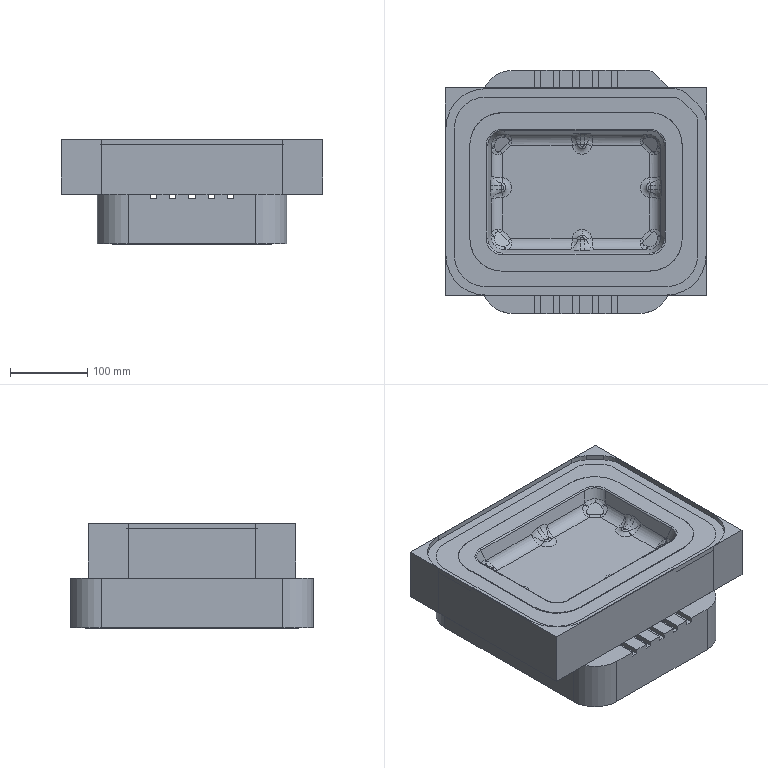NC program | NX | posted with a generic post | part box 339.125 x 315.125 x 135.5 mm
Lines 94253 to 95002 of 120728:
(B6 , TOOL : D10)
N188486 M6
N188488 G53
N188490 G17 G0 G90 X-147.735 Y117.398 S7000 M3 M8
N188492 G43 Z220.5 H0
N188494 Z66.
N188496 G94 G1 X-144.886 Y119.728 Z65.807 F4000.
N188498 X-141.056 Y122.268 Z65.566
N188500 X-136.99 Y124.414 Z65.325
N188502 X-132.732 Y126.144 Z65.084
N188504 X-128.321 Y127.44 Z64.844
N188506 X-123.804 Y128.29 Z64.603
N188508 X-119.224 Y128.685 Z64.362
N188510 X-112.322 Z64.
N188512 X126.349
N188514 G2 X141.199 Y122.534 R21.
N188516 G1 X157.412 Y106.321
N188518 G2 X163.563 Y91.472 R21.
N188520 G1 Y-82.685
N188522 G2 X117.563 Y-128.685 R46.
N188524 G1 X-117.563
N188526 G2 X-163.563 Y-82.685 R46.
N188528 G1 Y82.685
N188530 G2 X-117.563 Y128.685 R46.
N188532 G1 X-112.322
N188534 Y121.685
N188536 X126.349
N188538 G2 X136.249 Y117.584 R14.
N188540 G1 X152.462 Y101.371
N188542 G2 X156.563 Y91.472 R14.
N188544 G1 Y-82.685
N188546 G2 X117.563 Y-121.685 R39.
N188548 G1 X-117.563
N188550 G2 X-156.563 Y-82.685 R39.
N188552 G1 Y82.685
N188554 G2 X-117.563 Y121.685 R39.
N188556 G1 X-112.322
N188558 Y114.685
N188560 X126.349
N188562 G2 X131.299 Y112.635 R7.
N188564 G1 X147.512 Y96.422
N188566 G2 X149.563 Y91.472 R7.
N188568 G1 Y72.203
N188570 X142.563
N188572 G3 X138.153 Y83.687 R48.774
N188574 X118.341 Y103.394 R48.054
N188576 G1 X115.363 Y104.847
N188578 X115.273 Y104.887
N188580 X112.202 Y106.126
N188582 X112.11 Y106.159
N188584 X108.953 Y107.182
N188586 X108.858 Y107.209
N188588 X106.939 Y107.685
N188590 X126.349
N188592 X142.563 Y91.472
N188594 Y72.203
N188596 X143.501 Y67.292
N188598 G2 X143.963 Y60.543 R48.774
N188600 G1 Y-60.555
N188602 X143.962 Y-60.604
N188604 X143.85 Y-63.852
N188606 X143.843 Y-63.948
N188608 X143.51 Y-67.152
N188610 G2 X144.563 Y-67.479 R5.
N188612 G1 Y67.621
N188614 G2 X143.501 Y67.292 R5.
N188616 G1 X142.563 Y72.203
N188618 X149.563
N188620 Y-82.685
N188622 G2 X117.563 Y-114.685 R32.
N188624 G1 X107.081
N188626 Y-107.685
N188628 G3 X118.564 Y-103.276 R48.774
N188630 X138.272 Y-83.463 R48.054
N188632 G1 X139.725 Y-80.486
N188634 X139.765 Y-80.396
N188636 X141.003 Y-77.324
N188638 X141.037 Y-77.232
N188640 X142.059 Y-74.075
N188642 X142.086 Y-73.981
N188644 X142.563 Y-72.061
N188646 Y-82.685
N188648 G2 X117.563 Y-107.685 R25.
N188650 G1 X107.081
N188652 X102.17 Y-108.624
N188654 G2 X95.421 Y-109.085 R48.774
N188656 G1 X-95.433
N188658 X-95.481 Y-109.084
N188660 X-98.729 Y-108.972
N188662 X-98.826 Y-108.965
N188664 X-102.029 Y-108.633
N188666 G2 X-102.356 Y-109.685 R5.
N188668 G1 X102.498
N188670 G2 X102.17 Y-108.624 R5.
N188672 G1 X107.081 Y-107.685
N188674 Y-114.685
N188676 X-117.564
N188678 G2 X-149.563 Y-82.685 R32.
N188680 G1 Y-72.203
N188682 X-142.563
N188684 G3 X-138.153 Y-83.687 R48.774
N188686 X-118.341 Y-103.394 R48.054
N188688 G1 X-115.363 Y-104.847
N188690 X-115.273 Y-104.887
N188692 X-112.202 Y-106.126
N188694 X-112.11 Y-106.159
N188696 X-108.953 Y-107.182
N188698 X-108.858 Y-107.209
N188700 X-106.939 Y-107.685
N188702 X-117.565
N188704 G2 X-142.563 Y-82.685 R25.
N188706 G1 Y-72.203
N188708 X-149.563
N188710 Y82.685
N188712 G2 X-117.563 Y114.685 R32.
N188714 G1 X-112.322
N188716 Y107.685
N188718 X-107.081
N188720 X-102.17 Y108.624
N188722 G2 X-95.421 Y109.085 R48.774
N188724 G1 X95.433
N188726 X95.481 Y109.084
N188728 X98.729 Y108.972
N188730 X98.826 Y108.965
N188732 X102.029 Y108.633
N188734 G2 X102.356 Y109.685 R5.
N188736 G1 X-102.498
N188738 G2 X-102.17 Y108.624 R5.
N188740 G1 X-107.081 Y107.685
N188742 G3 X-118.564 Y103.276 R48.774
N188744 X-138.272 Y83.463 R48.054
N188746 G1 X-139.725 Y80.486
N188748 X-139.765 Y80.396
N188750 X-141.003 Y77.324
N188752 X-141.037 Y77.232
N188754 X-142.059 Y74.075
N188756 X-142.086 Y73.981
N188758 X-142.563 Y72.061
N188760 X-144.563 Y67.479
N188762 Y-67.621
N188764 G2 X-143.501 Y-67.292 R5.
N188766 X-143.963 Y-60.543 R48.774
N188768 G1 Y60.555
N188770 X-143.962 Y60.604
N188772 X-143.85 Y63.852
N188774 X-143.843 Y63.948
N188776 X-143.51 Y67.152
N188778 G2 X-144.563 Y67.479 R5.
N188780 G1 X-142.563 Y72.061
N188782 X-141.204 Y71.724
N188784 X-140.728 Y73.644
N188786 X-139.705 Y76.801
N188788 X-138.466 Y79.872
N188790 X-137.014 Y82.849
N188792 G2 X-117.902 Y102.042 R46.654
N188794 X-95.421 Y107.685 R47.374
N188796 G1 X95.433
N188798 G2 X117.727 Y102.136 R47.575
N188800 X136.92 Y83.024 R46.654
N188802 X142.563 Y60.543 R47.374
N188804 G1 Y-60.555
N188806 G2 X137.014 Y-82.849 R47.575
N188808 X117.902 Y-102.042 R46.654
N188810 X95.421 Y-107.685 R47.374
N188812 G1 X-95.433
N188814 G2 X-117.727 Y-102.136 R47.575
N188816 X-136.92 Y-83.024 R46.654
N188818 X-142.563 Y-60.543 R47.374
N188820 G1 Y60.555
N188822 X-142.45 Y63.803
N188824 X-142.106 Y67.115
N188826 X-141.531 Y70.403
N188828 X-141.204 Y71.724
N188830 X-142.563 Y72.061
N188832 Y82.685
N188834 G2 X-117.563 Y107.685 R25.
N188836 G1 X-112.322
N188838 G3 X-110.322 Y109.685 R2.
N188840 G1 Z65.
N188842 G0 Z220.5
(B7 , TOOL : D10)
N188844 X-108.451 Y-127.685
N188846 Z65.
N188848 G1 X-119.206 Z64.991
N188850 X-123.684 Y-127.297 Z64.987
N188852 X-128.1 Y-126.465 Z64.983
N188854 X-132.412 Y-125.196 Z64.979
N188856 X-136.576 Y-123.504 Z64.975
N188858 X-140.55 Y-121.405 Z64.971
N188860 X-144.296 Y-118.921 Z64.967
N188862 X-147.775 Y-116.075 Z64.963
N188864 X-150.953 Y-112.897 Z64.959
N188866 X-153.798 Y-109.418 Z64.955
N188868 X-156.283 Y-105.673 Z64.951
N188870 X-158.381 Y-101.698 Z64.947
N188872 X-160.074 Y-97.535 Z64.944
N188874 X-161.342 Y-93.223 Z64.94
N188876 X-162.175 Y-88.806 Z64.936
N188878 X-162.563 Y-84.328 Z64.932
N188880 Y84.328 Z64.785
N188882 X-162.175 Y88.806 Z64.781
N188884 X-161.342 Y93.223 Z64.777
N188886 X-160.074 Y97.535 Z64.773
N188888 X-158.381 Y101.698 Z64.769
N188890 X-156.283 Y105.673 Z64.765
N188892 X-153.798 Y109.418 Z64.761
N188894 X-150.953 Y112.897 Z64.757
N188896 X-147.775 Y116.075 Z64.753
N188898 X-144.296 Y118.921 Z64.749
N188900 X-140.55 Y121.405 Z64.745
N188902 X-136.576 Y123.504 Z64.741
N188904 X-132.412 Y125.196 Z64.738
N188906 X-128.1 Y126.465 Z64.734
N188908 X-123.684 Y127.297 Z64.73
N188910 X-119.206 Y127.685 Z64.726
N188912 X127.445 Z64.511
N188914 X130.131 Y127.355 Z64.508
N188916 X132.747 Y126.666 Z64.506
N188918 X135.247 Y125.63 Z64.503
N188920 X137.584 Y124.267 Z64.501
N188922 X139.717 Y122.602 Z64.499
N188924 X157.48 Y104.839 Z64.477
N188926 X159.145 Y102.707 Z64.474
N188928 X160.508 Y100.369 Z64.472
N188930 X161.543 Y97.87 Z64.47
N188932 X162.232 Y95.253 Z64.467
N188934 X162.563 Y92.568 Z64.465
N188936 Y-84.328 Z64.311
N188938 X162.175 Y-88.806 Z64.307
N188940 X161.342 Y-93.223 Z64.303
N188942 X160.074 Y-97.535 Z64.299
N188944 X158.381 Y-101.698 Z64.295
N188946 X156.283 Y-105.673 Z64.291
N188948 X153.798 Y-109.418 Z64.287
N188950 X150.953 Y-112.897 Z64.283
N188952 X147.775 Y-116.075 Z64.279
N188954 X144.296 Y-118.921 Z64.275
N188956 X140.55 Y-121.405 Z64.271
N188958 X136.576 Y-123.504 Z64.267
N188960 X132.412 Y-125.196 Z64.264
N188962 X128.1 Y-126.465 Z64.26
N188964 X123.684 Y-127.297 Z64.256
N188966 X119.206 Y-127.685 Z64.252
N188968 X-119.206 Z64.044
N188970 X-123.684 Y-127.297 Z64.04
N188972 X-128.1 Y-126.465 Z64.036
N188974 X-132.412 Y-125.196 Z64.032
N188976 X-136.576 Y-123.504 Z64.028
N188978 X-140.55 Y-121.405 Z64.024
N188980 X-144.296 Y-118.921 Z64.02
N188982 X-147.775 Y-116.075 Z64.016
N188984 X-150.953 Y-112.897 Z64.012
N188986 X-153.798 Y-109.418 Z64.008
N188988 X-156.283 Y-105.673 Z64.005
N188990 X-158.381 Y-101.698 Z64.001
N188992 X-160.074 Y-97.535 Z63.997
N188994 X-161.342 Y-93.223 Z63.993
N188996 X-162.175 Y-88.806 Z63.989
N188998 X-162.563 Y-84.328 Z63.985
N189000 Y84.328 Z63.838
N189002 X-162.175 Y88.806 Z63.834
N189004 X-161.342 Y93.223 Z63.83
N189006 X-160.074 Y97.535 Z63.826
N189008 X-158.381 Y101.698 Z63.822
N189010 X-156.283 Y105.673 Z63.818
N189012 X-153.798 Y109.418 Z63.814
N189014 X-150.953 Y112.897 Z63.81
N189016 X-147.775 Y116.075 Z63.806
N189018 X-144.296 Y118.921 Z63.802
N189020 X-140.55 Y121.405 Z63.798
N189022 X-136.576 Y123.504 Z63.795
N189024 X-132.412 Y125.196 Z63.791
N189026 X-128.1 Y126.465 Z63.787
N189028 X-123.684 Y127.297 Z63.783
N189030 X-119.206 Y127.685 Z63.779
N189032 X127.445 Z63.564
N189034 X130.131 Y127.355 Z63.561
N189036 X132.747 Y126.666 Z63.559
N189038 X135.247 Y125.63 Z63.557
N189040 X137.584 Y124.267 Z63.554
N189042 X139.717 Y122.602 Z63.552
N189044 X157.48 Y104.839 Z63.53
N189046 X159.145 Y102.707 Z63.528
N189048 X160.508 Y100.369 Z63.525
N189050 X161.543 Y97.87 Z63.523
N189052 X162.232 Y95.253 Z63.52
N189054 X162.563 Y92.568 Z63.518
N189056 Y-84.328 Z63.364
N189058 X162.175 Y-88.806 Z63.36
N189060 X161.342 Y-93.223 Z63.356
N189062 X160.074 Y-97.535 Z63.352
N189064 X158.381 Y-101.698 Z63.348
N189066 X156.283 Y-105.673 Z63.344
N189068 X153.798 Y-109.418 Z63.34
N189070 X150.953 Y-112.897 Z63.336
N189072 X147.775 Y-116.075 Z63.332
N189074 X144.296 Y-118.921 Z63.328
N189076 X140.55 Y-121.405 Z63.325
N189078 X136.576 Y-123.504 Z63.321
N189080 X132.412 Y-125.196 Z63.317
N189082 X128.1 Y-126.465 Z63.313
N189084 X123.684 Y-127.297 Z63.309
N189086 X119.206 Y-127.685 Z63.305
N189088 X-119.206 Z63.097
N189090 X-123.684 Y-127.297 Z63.093
N189092 X-128.1 Y-126.465 Z63.089
N189094 X-132.412 Y-125.196 Z63.085
N189096 X-136.576 Y-123.504 Z63.081
N189098 X-140.55 Y-121.405 Z63.077
N189100 X-144.296 Y-118.921 Z63.073
N189102 X-147.775 Y-116.075 Z63.069
N189104 X-150.953 Y-112.897 Z63.065
N189106 X-153.798 Y-109.418 Z63.062
N189108 X-156.283 Y-105.673 Z63.058
N189110 X-158.381 Y-101.698 Z63.054
N189112 X-160.074 Y-97.535 Z63.05
N189114 X-161.342 Y-93.223 Z63.046
N189116 X-162.175 Y-88.806 Z63.042
N189118 X-162.563 Y-84.328 Z63.038
N189120 Y84.328 Z62.891
N189122 X-162.175 Y88.806 Z62.887
N189124 X-161.342 Y93.223 Z62.883
N189126 X-160.074 Y97.535 Z62.879
N189128 X-158.381 Y101.698 Z62.875
N189130 X-156.283 Y105.673 Z62.871
N189132 X-153.798 Y109.418 Z62.867
N189134 X-150.953 Y112.897 Z62.863
N189136 X-147.775 Y116.075 Z62.859
N189138 X-144.296 Y118.921 Z62.856
N189140 X-140.55 Y121.405 Z62.852
N189142 X-136.576 Y123.504 Z62.848
N189144 X-132.412 Y125.196 Z62.844
N189146 X-128.1 Y126.465 Z62.84
N189148 X-123.684 Y127.297 Z62.836
N189150 X-119.206 Y127.685 Z62.832
N189152 X127.445 Z62.617
N189154 X130.131 Y127.355 Z62.614
N189156 X132.747 Y126.666 Z62.612
N189158 X135.247 Y125.63 Z62.61
N189160 X137.584 Y124.267 Z62.607
N189162 X139.717 Y122.602 Z62.605
N189164 X157.48 Y104.839 Z62.583
N189166 X159.145 Y102.707 Z62.581
N189168 X160.508 Y100.369 Z62.578
N189170 X161.543 Y97.87 Z62.576
N189172 X162.232 Y95.253 Z62.574
N189174 X162.563 Y92.568 Z62.571
N189176 Y-84.328 Z62.417
N189178 X162.175 Y-88.806 Z62.413
N189180 X161.342 Y-93.223 Z62.409
N189182 X160.074 Y-97.535 Z62.405
N189184 X158.381 Y-101.698 Z62.401
N189186 X156.283 Y-105.673 Z62.397
N189188 X153.798 Y-109.418 Z62.393
N189190 X150.953 Y-112.897 Z62.389
N189192 X147.775 Y-116.075 Z62.385
N189194 X144.296 Y-118.921 Z62.382
N189196 X140.55 Y-121.405 Z62.378
N189198 X136.576 Y-123.504 Z62.374
N189200 X132.412 Y-125.196 Z62.37
N189202 X128.1 Y-126.465 Z62.366
N189204 X123.684 Y-127.297 Z62.362
N189206 X119.206 Y-127.685 Z62.358
N189208 X-119.206 Z62.15
N189210 X-123.684 Y-127.297 Z62.146
N189212 X-128.1 Y-126.465 Z62.142
N189214 X-132.412 Y-125.196 Z62.138
N189216 X-136.576 Y-123.504 Z62.134
N189218 X-140.55 Y-121.405 Z62.13
N189220 X-144.296 Y-118.921 Z62.126
N189222 X-147.775 Y-116.075 Z62.123
N189224 X-150.953 Y-112.897 Z62.119
N189226 X-153.798 Y-109.418 Z62.115
N189228 X-156.283 Y-105.673 Z62.111
N189230 X-158.381 Y-101.698 Z62.107
N189232 X-160.074 Y-97.535 Z62.103
N189234 X-161.342 Y-93.223 Z62.099
N189236 X-162.175 Y-88.806 Z62.095
N189238 X-162.563 Y-84.328 Z62.091
N189240 Y84.328 Z61.944
N189242 X-162.175 Y88.806 Z61.94
N189244 X-161.342 Y93.223 Z61.936
N189246 X-160.074 Y97.535 Z61.932
N189248 X-158.381 Y101.698 Z61.928
N189250 X-156.283 Y105.673 Z61.924
N189252 X-153.798 Y109.418 Z61.92
N189254 X-150.953 Y112.897 Z61.917
N189256 X-147.775 Y116.075 Z61.913
N189258 X-144.296 Y118.921 Z61.909
N189260 X-140.55 Y121.405 Z61.905
N189262 X-136.576 Y123.504 Z61.901
N189264 X-132.412 Y125.196 Z61.897
N189266 X-128.1 Y126.465 Z61.893
N189268 X-123.684 Y127.297 Z61.889
N189270 X-119.206 Y127.685 Z61.885
N189272 X127.445 Z61.67
N189274 X130.131 Y127.355 Z61.668
N189276 X132.747 Y126.666 Z61.665
N189278 X135.247 Y125.63 Z61.663
N189280 X137.584 Y124.267 Z61.66
N189282 X139.717 Y122.602 Z61.658
N189284 X157.48 Y104.839 Z61.636
N189286 X159.145 Y102.707 Z61.634
N189288 X160.508 Y100.369 Z61.631
N189290 X161.543 Y97.87 Z61.629
N189292 X162.232 Y95.253 Z61.627
N189294 X162.563 Y92.568 Z61.624
N189296 Y-84.328 Z61.47
N189298 X162.175 Y-88.806 Z61.466
N189300 X161.342 Y-93.223 Z61.462
N189302 X160.074 Y-97.535 Z61.458
N189304 X158.381 Y-101.698 Z61.454
N189306 X156.283 Y-105.673 Z61.45
N189308 X153.798 Y-109.418 Z61.446
N189310 X150.953 Y-112.897 Z61.443
N189312 X147.775 Y-116.075 Z61.439
N189314 X144.296 Y-118.921 Z61.435
N189316 X140.55 Y-121.405 Z61.431
N189318 X136.576 Y-123.504 Z61.427
N189320 X132.412 Y-125.196 Z61.423
N189322 X128.1 Y-126.465 Z61.419
N189324 X123.684 Y-127.297 Z61.415
N189326 X119.206 Y-127.685 Z61.411
N189328 X-119.206 Z61.203
N189330 X-123.684 Y-127.297 Z61.199
N189332 X-128.1 Y-126.465 Z61.195
N189334 X-132.412 Y-125.196 Z61.191
N189336 X-136.576 Y-123.504 Z61.187
N189338 X-140.55 Y-121.405 Z61.183
N189340 X-144.296 Y-118.921 Z61.18
N189342 X-147.775 Y-116.075 Z61.176
N189344 X-150.953 Y-112.897 Z61.172
N189346 X-153.798 Y-109.418 Z61.168
N189348 X-156.283 Y-105.673 Z61.164
N189350 X-158.381 Y-101.698 Z61.16
N189352 X-160.074 Y-97.535 Z61.156
N189354 X-161.342 Y-93.223 Z61.152
N189356 X-162.175 Y-88.806 Z61.148
N189358 X-162.563 Y-84.328 Z61.144
N189360 Y84.328 Z60.997
N189362 X-162.175 Y88.806 Z60.993
N189364 X-161.342 Y93.223 Z60.989
N189366 X-160.074 Y97.535 Z60.985
N189368 X-158.381 Y101.698 Z60.981
N189370 X-156.283 Y105.673 Z60.977
N189372 X-153.798 Y109.418 Z60.974
N189374 X-150.953 Y112.897 Z60.97
N189376 X-147.775 Y116.075 Z60.966
N189378 X-144.296 Y118.921 Z60.962
N189380 X-140.55 Y121.405 Z60.958
N189382 X-136.576 Y123.504 Z60.954
N189384 X-132.412 Y125.196 Z60.95
N189386 X-128.1 Y126.465 Z60.946
N189388 X-123.684 Y127.297 Z60.942
N189390 X-119.206 Y127.685 Z60.938
N189392 X127.445 Z60.723
N189394 X130.131 Y127.355 Z60.721
N189396 X132.747 Y126.666 Z60.718
N189398 X135.247 Y125.63 Z60.716
N189400 X137.584 Y124.267 Z60.714
N189402 X139.717 Y122.602 Z60.711
N189404 X157.48 Y104.839 Z60.689
N189406 X159.145 Y102.707 Z60.687
N189408 X160.508 Y100.369 Z60.685
N189410 X161.543 Y97.87 Z60.682
N189412 X162.232 Y95.253 Z60.68
N189414 X162.563 Y92.568 Z60.677
N189416 Y-84.328 Z60.523
N189418 X162.175 Y-88.806 Z60.519
N189420 X161.342 Y-93.223 Z60.515
N189422 X160.074 Y-97.535 Z60.511
N189424 X158.381 Y-101.698 Z60.507
N189426 X156.283 Y-105.673 Z60.503
N189428 X153.798 Y-109.418 Z60.5
N189430 X150.953 Y-112.897 Z60.496
N189432 X147.775 Y-116.075 Z60.492
N189434 X144.296 Y-118.921 Z60.488
N189436 X140.55 Y-121.405 Z60.484
N189438 X136.576 Y-123.504 Z60.48
N189440 X132.412 Y-125.196 Z60.476
N189442 X128.1 Y-126.465 Z60.472
N189444 X123.684 Y-127.297 Z60.468
N189446 X119.206 Y-127.685 Z60.464
N189448 X-119.206 Z60.256
N189450 X-123.684 Y-127.297 Z60.252
N189452 X-128.1 Y-126.465 Z60.248
N189454 X-132.412 Y-125.196 Z60.244
N189456 X-136.576 Y-123.504 Z60.241
N189458 X-140.55 Y-121.405 Z60.237
N189460 X-144.296 Y-118.921 Z60.233
N189462 X-147.775 Y-116.075 Z60.229
N189464 X-150.953 Y-112.897 Z60.225
N189466 X-153.798 Y-109.418 Z60.221
N189468 X-156.283 Y-105.673 Z60.217
N189470 X-158.381 Y-101.698 Z60.213
N189472 X-160.074 Y-97.535 Z60.209
N189474 X-161.342 Y-93.223 Z60.205
N189476 X-162.175 Y-88.806 Z60.201
N189478 X-162.563 Y-84.328 Z60.197
N189480 Y84.328 Z60.05
N189482 X-162.175 Y88.806 Z60.046
N189484 X-161.342 Y93.223 Z60.042
N189486 X-160.074 Y97.535 Z60.038
N189488 X-158.381 Y101.698 Z60.035
N189490 X-156.283 Y105.673 Z60.031
N189492 X-153.798 Y109.418 Z60.027
N189494 X-150.953 Y112.897 Z60.023
N189496 X-147.775 Y116.075 Z60.019
N189498 X-144.296 Y118.921 Z60.015
N189500 X-140.55 Y121.405 Z60.011
N189502 X-136.576 Y123.504 Z60.007
N189504 X-132.412 Y125.196 Z60.003
N189506 X-128.1 Y126.465 Z59.999
N189508 X-123.684 Y127.297 Z59.995
N189510 X-119.206 Y127.685 Z59.991
N189512 X127.445 Z59.776
N189514 X130.131 Y127.355 Z59.774
N189516 X132.747 Y126.666 Z59.771
N189518 X135.247 Y125.63 Z59.769
N189520 X137.584 Y124.267 Z59.767
N189522 X139.717 Y122.602 Z59.764
N189524 X157.48 Y104.839 Z59.742
N189526 X159.145 Y102.707 Z59.74
N189528 X160.508 Y100.369 Z59.738
N189530 X161.543 Y97.87 Z59.735
N189532 X162.232 Y95.253 Z59.733
N189534 X162.563 Y92.568 Z59.731
N189536 Y-84.328 Z59.576
N189538 X162.175 Y-88.806 Z59.572
N189540 X161.342 Y-93.223 Z59.568
N189542 X160.074 Y-97.535 Z59.564
N189544 X158.381 Y-101.698 Z59.561
N189546 X156.283 Y-105.673 Z59.557
N189548 X153.798 Y-109.418 Z59.553
N189550 X150.953 Y-112.897 Z59.549
N189552 X147.775 Y-116.075 Z59.545
N189554 X144.296 Y-118.921 Z59.541
N189556 X140.55 Y-121.405 Z59.537
N189558 X136.576 Y-123.504 Z59.533
N189560 X132.412 Y-125.196 Z59.529
N189562 X128.1 Y-126.465 Z59.525
N189564 X123.684 Y-127.297 Z59.521
N189566 X119.206 Y-127.685 Z59.517
N189568 X-119.206 Z59.309
N189570 X-123.684 Y-127.297 Z59.305
N189572 X-128.1 Y-126.465 Z59.301
N189574 X-132.412 Y-125.196 Z59.298
N189576 X-136.576 Y-123.504 Z59.294
N189578 X-140.55 Y-121.405 Z59.29
N189580 X-144.296 Y-118.921 Z59.286
N189582 X-147.775 Y-116.075 Z59.282
N189584 X-150.953 Y-112.897 Z59.278
N189586 X-153.798 Y-109.418 Z59.274
N189588 X-156.283 Y-105.673 Z59.27
N189590 X-158.381 Y-101.698 Z59.266
N189592 X-160.074 Y-97.535 Z59.262
N189594 X-161.342 Y-93.223 Z59.258
N189596 X-162.175 Y-88.806 Z59.254
N189598 X-162.563 Y-84.328 Z59.25
N189600 Y84.328 Z59.103
N189602 X-162.175 Y88.806 Z59.099
N189604 X-161.342 Y93.223 Z59.095
N189606 X-160.074 Y97.535 Z59.092
N189608 X-158.381 Y101.698 Z59.088
N189610 X-156.283 Y105.673 Z59.084
N189612 X-153.798 Y109.418 Z59.08
N189614 X-150.953 Y112.897 Z59.076
N189616 X-147.775 Y116.075 Z59.072
N189618 X-144.296 Y118.921 Z59.068
N189620 X-140.55 Y121.405 Z59.064
N189622 X-136.576 Y123.504 Z59.06
N189624 X-132.412 Y125.196 Z59.056
N189626 X-128.1 Y126.465 Z59.052
N189628 X-123.684 Y127.297 Z59.048
N189630 X-119.206 Y127.685 Z59.044
N189632 X127.445 Z58.829
N189634 X130.131 Y127.355 Z58.827
N189636 X132.747 Y126.666 Z58.825
N189638 X135.247 Y125.63 Z58.822
N189640 X137.584 Y124.267 Z58.82
N189642 X139.717 Y122.602 Z58.817
N189644 X157.48 Y104.839 Z58.796
N189646 X159.145 Y102.707 Z58.793
N189648 X160.508 Y100.369 Z58.791
N189650 X161.543 Y97.87 Z58.788
N189652 X162.232 Y95.253 Z58.786
N189654 X162.563 Y92.568 Z58.784
N189656 Y-84.328 Z58.629
N189658 X162.175 Y-88.806 Z58.625
N189660 X161.342 Y-93.223 Z58.621
N189662 X160.074 Y-97.535 Z58.618
N189664 X158.381 Y-101.698 Z58.614
N189666 X156.283 Y-105.673 Z58.61
N189668 X153.798 Y-109.418 Z58.606
N189670 X150.953 Y-112.897 Z58.602
N189672 X147.775 Y-116.075 Z58.598
N189674 X144.296 Y-118.921 Z58.594
N189676 X140.55 Y-121.405 Z58.59
N189678 X136.576 Y-123.504 Z58.586
N189680 X132.412 Y-125.196 Z58.582
N189682 X128.1 Y-126.465 Z58.578
N189684 X123.684 Y-127.297 Z58.574
N189686 X119.206 Y-127.685 Z58.571
N189688 X-119.206 Z58.362
N189690 X-123.684 Y-127.297 Z58.359
N189692 X-128.1 Y-126.465 Z58.355
N189694 X-132.412 Y-125.196 Z58.351
N189696 X-136.576 Y-123.504 Z58.347
N189698 X-140.55 Y-121.405 Z58.343
N189700 X-144.296 Y-118.921 Z58.339
N189702 X-147.775 Y-116.075 Z58.335
N189704 X-150.953 Y-112.897 Z58.331
N189706 X-153.798 Y-109.418 Z58.327
N189708 X-156.283 Y-105.673 Z58.323
N189710 X-158.381 Y-101.698 Z58.319
N189712 X-160.074 Y-97.535 Z58.315
N189714 X-161.342 Y-93.223 Z58.311
N189716 X-162.175 Y-88.806 Z58.308
N189718 X-162.563 Y-84.328 Z58.304
N189720 Y84.328 Z58.156
N189722 X-162.175 Y88.806 Z58.153
N189724 X-161.342 Y93.223 Z58.149
N189726 X-160.074 Y97.535 Z58.145
N189728 X-158.381 Y101.698 Z58.141
N189730 X-156.283 Y105.673 Z58.137
N189732 X-153.798 Y109.418 Z58.133
N189734 X-150.953 Y112.897 Z58.129
N189736 X-147.775 Y116.075 Z58.125
N189738 X-144.296 Y118.921 Z58.121
N189740 X-140.55 Y121.405 Z58.117
N189742 X-136.576 Y123.504 Z58.113
N189744 X-132.412 Y125.196 Z58.109
N189746 X-128.1 Y126.465 Z58.105
N189748 X-123.684 Y127.297 Z58.102
N189750 X-119.206 Y127.685 Z58.098
N189752 X127.445 Z57.882
N189754 X130.131 Y127.355 Z57.88
N189756 X132.747 Y126.666 Z57.878
N189758 X135.247 Y125.63 Z57.875
N189760 X137.584 Y124.267 Z57.873
N189762 X139.717 Y122.602 Z57.871
N189764 X157.48 Y104.839 Z57.849
N189766 X159.145 Y102.707 Z57.846
N189768 X160.508 Y100.369 Z57.844
N189770 X161.543 Y97.87 Z57.842
N189772 X162.232 Y95.253 Z57.839
N189774 X162.563 Y92.568 Z57.837
N189776 Y-84.328 Z57.682
N189778 X162.175 Y-88.806 Z57.679
N189780 X161.342 Y-93.223 Z57.675
N189782 X160.074 Y-97.535 Z57.671
N189784 X158.381 Y-101.698 Z57.667
N189786 X156.283 Y-105.673 Z57.663
N189788 X153.798 Y-109.418 Z57.659
N189790 X150.953 Y-112.897 Z57.655
N189792 X147.775 Y-116.075 Z57.651
N189794 X144.296 Y-118.921 Z57.647
N189796 X140.55 Y-121.405 Z57.643
N189798 X136.576 Y-123.504 Z57.639
N189800 X132.412 Y-125.196 Z57.635
N189802 X128.1 Y-126.465 Z57.631
N189804 X123.684 Y-127.297 Z57.628
N189806 X119.206 Y-127.685 Z57.624
N189808 X-119.206 Z57.416
N189810 X-123.684 Y-127.297 Z57.412
N189812 X-128.1 Y-126.465 Z57.408
N189814 X-132.412 Y-125.196 Z57.404
N189816 X-136.576 Y-123.504 Z57.4
N189818 X-140.55 Y-121.405 Z57.396
N189820 X-144.296 Y-118.921 Z57.392
N189822 X-147.775 Y-116.075 Z57.388
N189824 X-150.953 Y-112.897 Z57.384
N189826 X-153.798 Y-109.418 Z57.38
N189828 X-156.283 Y-105.673 Z57.376
N189830 X-158.381 Y-101.698 Z57.372
N189832 X-160.074 Y-97.535 Z57.369
N189834 X-161.342 Y-93.223 Z57.365
N189836 X-162.175 Y-88.806 Z57.361
N189838 X-162.563 Y-84.328 Z57.357
N189840 Y84.328 Z57.21
N189842 X-162.175 Y88.806 Z57.206
N189844 X-161.342 Y93.223 Z57.202
N189846 X-160.074 Y97.535 Z57.198
N189848 X-158.381 Y101.698 Z57.194
N189850 X-156.283 Y105.673 Z57.19
N189852 X-153.798 Y109.418 Z57.186
N189854 X-150.953 Y112.897 Z57.182
N189856 X-147.775 Y116.075 Z57.178
N189858 X-144.296 Y118.921 Z57.174
N189860 X-140.55 Y121.405 Z57.17
N189862 X-136.576 Y123.504 Z57.166
N189864 X-132.412 Y125.196 Z57.162
N189866 X-128.1 Y126.465 Z57.159
N189868 X-123.684 Y127.297 Z57.155
N189870 X-119.206 Y127.685 Z57.151
N189872 X127.445 Z56.935
N189874 X130.131 Y127.355 Z56.933
N189876 X132.747 Y126.666 Z56.931
N189878 X135.247 Y125.63 Z56.928
N189880 X137.584 Y124.267 Z56.926
N189882 X139.717 Y122.602 Z56.924
N189884 X157.48 Y104.839 Z56.902
N189886 X159.145 Y102.707 Z56.899
N189888 X160.508 Y100.369 Z56.897
N189890 X161.543 Y97.87 Z56.895
N189892 X162.232 Y95.253 Z56.892
N189894 X162.563 Y92.568 Z56.89
N189896 Y-84.328 Z56.736
N189898 X162.175 Y-88.806 Z56.732
N189900 X161.342 Y-93.223 Z56.728
N189902 X160.074 Y-97.535 Z56.724
N189904 X158.381 Y-101.698 Z56.72
N189906 X156.283 Y-105.673 Z56.716
N189908 X153.798 Y-109.418 Z56.712
N189910 X150.953 Y-112.897 Z56.708
N189912 X147.775 Y-116.075 Z56.704
N189914 X144.296 Y-118.921 Z56.7
N189916 X140.55 Y-121.405 Z56.696
N189918 X136.576 Y-123.504 Z56.692
N189920 X132.412 Y-125.196 Z56.689
N189922 X128.1 Y-126.465 Z56.685
N189924 X123.684 Y-127.297 Z56.681
N189926 X119.206 Y-127.685 Z56.677
N189928 X-119.206 Z56.469
N189930 X-123.684 Y-127.297 Z56.465
N189932 X-128.1 Y-126.465 Z56.461
N189934 X-132.412 Y-125.196 Z56.457
N189936 X-136.576 Y-123.504 Z56.453
N189938 X-140.55 Y-121.405 Z56.449
N189940 X-144.296 Y-118.921 Z56.445
N189942 X-147.775 Y-116.075 Z56.441
N189944 X-150.953 Y-112.897 Z56.437
N189946 X-153.798 Y-109.418 Z56.433
N189948 X-156.283 Y-105.673 Z56.429
N189950 X-158.381 Y-101.698 Z56.426
N189952 X-160.074 Y-97.535 Z56.422
N189954 X-161.342 Y-93.223 Z56.418
N189956 X-162.175 Y-88.806 Z56.414
N189958 X-162.563 Y-84.328 Z56.41
N189960 Y84.328 Z56.263
N189962 X-162.175 Y88.806 Z56.259
N189964 X-161.342 Y93.223 Z56.255
N189966 X-160.074 Y97.535 Z56.251
N189968 X-158.381 Y101.698 Z56.247
N189970 X-156.283 Y105.673 Z56.243
N189972 X-153.798 Y109.418 Z56.239